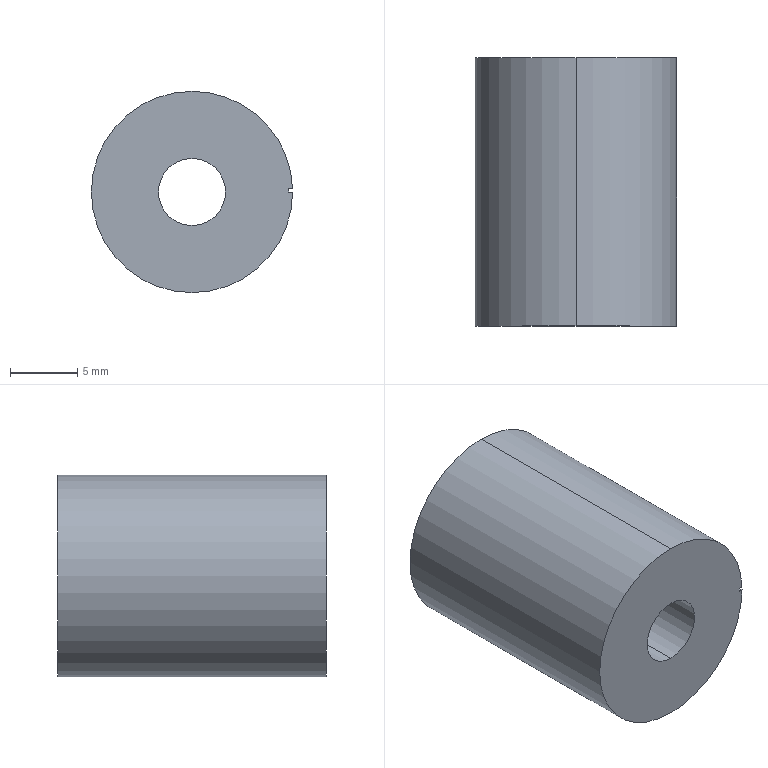Part | SolidWorks | features Extrusion 1, ICE 1 | 1 solid | 10 faces | box 15 x 20 x 15 mm | volume 3140 mm3 | cylinder 5 | plane 5 | commonest cylinder face diameters 15 x3 5 x2
STEP:
#1=CARTESIAN_POINT('',(0.,20.,-2.5));
#2=VERTEX_POINT('',#1);
#3=CARTESIAN_POINT('',(0.,20.,2.5));
#4=VERTEX_POINT('',#3);
#5=CARTESIAN_POINT('',(0.,20.,0.));
#6=DIRECTION('',(0.,1.,0.));
#7=DIRECTION('',(0.,0.,1.));
#8=AXIS2_PLACEMENT_3D('',#5,#6,#7);
#9=CIRCLE('',#8,2.5);
#10=EDGE_CURVE('',#2,#4,#9,.T.);
#11=ORIENTED_EDGE('',*,*,#10,.T.);
#12=CARTESIAN_POINT('',(0.,0.,2.5));
#13=VERTEX_POINT('',#12);
#14=CARTESIAN_POINT('',(0.,20.,2.5));
#15=DIRECTION('',(0.,-1.,0.));
#16=VECTOR('',#15,1000.);
#17=LINE('',#14,#16);
#18=EDGE_CURVE('',#4,#13,#17,.T.);
#19=ORIENTED_EDGE('',*,*,#18,.T.);
#20=CARTESIAN_POINT('',(0.,0.,-2.5));
#21=VERTEX_POINT('',#20);
#22=CARTESIAN_POINT('',(0.,0.,0.));
#23=DIRECTION('',(0.,1.,0.));
#24=DIRECTION('',(0.,0.,1.));
#25=AXIS2_PLACEMENT_3D('',#22,#23,#24);
#26=CIRCLE('',#25,2.5);
#27=EDGE_CURVE('',#21,#13,#26,.T.);
#28=ORIENTED_EDGE('',*,*,#27,.F.);
#29=CARTESIAN_POINT('',(0.,20.,-2.5));
#30=DIRECTION('',(0.,-1.,0.));
#31=VECTOR('',#30,1000.);
#32=LINE('',#29,#31);
#33=EDGE_CURVE('',#2,#21,#32,.T.);
#34=ORIENTED_EDGE('',*,*,#33,.F.);
#35=EDGE_LOOP('',(#11,#19,#28,#34));
#36=FACE_OUTER_BOUND('',#35,.T.);
#37=CARTESIAN_POINT('',(0.,20.,0.));
#38=DIRECTION('',(0.,-1.,0.));
#39=DIRECTION('',(0.,0.,-1.));
#40=AXIS2_PLACEMENT_3D('',#37,#38,#39);
#41=CYLINDRICAL_SURFACE('',#40,2.5);
#42=ADVANCED_FACE('',(#36),#41,.F.);
#43=CARTESIAN_POINT('',(0.,20.,7.5));
#44=VERTEX_POINT('',#43);
#45=CARTESIAN_POINT('',(7.496,20.,0.2452));
#46=VERTEX_POINT('',#45);
#47=CARTESIAN_POINT('',(0.,20.,0.));
#48=DIRECTION('',(0.,1.,0.));
#49=DIRECTION('',(0.,0.,1.));
#50=AXIS2_PLACEMENT_3D('',#47,#48,#49);
#51=CIRCLE('',#50,7.5);
#52=EDGE_CURVE('',#44,#46,#51,.T.);
#53=ORIENTED_EDGE('',*,*,#52,.F.);
#54=CARTESIAN_POINT('',(0.,0.,7.5));
#55=VERTEX_POINT('',#54);
#56=CARTESIAN_POINT('',(0.,20.,7.5));
#57=DIRECTION('',(0.,-1.,0.));
#58=VECTOR('',#57,1000.);
#59=LINE('',#56,#58);
#60=EDGE_CURVE('',#44,#55,#59,.T.);
#61=ORIENTED_EDGE('',*,*,#60,.T.);
#62=CARTESIAN_POINT('',(7.496,0.,0.2452));
#63=VERTEX_POINT('',#62);
#64=CARTESIAN_POINT('',(0.,0.,0.));
#65=DIRECTION('',(0.,1.,0.));
#66=DIRECTION('',(0.,0.,1.));
#67=AXIS2_PLACEMENT_3D('',#64,#65,#66);
#68=CIRCLE('',#67,7.5);
#69=EDGE_CURVE('',#55,#63,#68,.T.);
#70=ORIENTED_EDGE('',*,*,#69,.T.);
#71=CARTESIAN_POINT('',(7.496,20.,0.2452));
#72=DIRECTION('',(0.,1.,0.));
#73=VECTOR('',#72,1000.);
#74=LINE('',#71,#73);
#75=EDGE_CURVE('',#63,#46,#74,.T.);
#76=ORIENTED_EDGE('',*,*,#75,.T.);
#77=EDGE_LOOP('',(#53,#61,#70,#76));
#78=FACE_OUTER_BOUND('',#77,.T.);
#79=CARTESIAN_POINT('',(0.,20.,0.));
#80=DIRECTION('',(0.,-1.,0.));
#81=DIRECTION('',(0.,0.,-1.));
#82=AXIS2_PLACEMENT_3D('',#79,#80,#81);
#83=CYLINDRICAL_SURFACE('',#82,7.5);
#84=ADVANCED_FACE('',(#78),#83,.T.);
#85=ORIENTED_EDGE('',*,*,#60,.F.);
#86=CARTESIAN_POINT('',(0.,20.,-7.5));
#87=VERTEX_POINT('',#86);
#88=CARTESIAN_POINT('',(0.,20.,0.));
#89=DIRECTION('',(0.,1.,0.));
#90=DIRECTION('',(0.,0.,1.));
#91=AXIS2_PLACEMENT_3D('',#88,#89,#90);
#92=CIRCLE('',#91,7.5);
#93=EDGE_CURVE('',#87,#44,#92,.T.);
#94=ORIENTED_EDGE('',*,*,#93,.F.);
#95=CARTESIAN_POINT('',(0.,0.,-7.5));
#96=VERTEX_POINT('',#95);
#97=CARTESIAN_POINT('',(0.,20.,-7.5));
#98=DIRECTION('',(0.,-1.,0.));
#99=VECTOR('',#98,1000.);
#100=LINE('',#97,#99);
#101=EDGE_CURVE('',#87,#96,#100,.T.);
#102=ORIENTED_EDGE('',*,*,#101,.T.);
#103=CARTESIAN_POINT('',(0.,0.,0.));
#104=DIRECTION('',(0.,1.,0.));
#105=DIRECTION('',(0.,0.,1.));
#106=AXIS2_PLACEMENT_3D('',#103,#104,#105);
#107=CIRCLE('',#106,7.5);
#108=EDGE_CURVE('',#96,#55,#107,.T.);
#109=ORIENTED_EDGE('',*,*,#108,.T.);
#110=EDGE_LOOP('',(#85,#94,#102,#109));
#111=FACE_OUTER_BOUND('',#110,.T.);
#112=CARTESIAN_POINT('',(0.,20.,0.));
#113=DIRECTION('',(0.,-1.,0.));
#114=DIRECTION('',(0.,0.,-1.));
#115=AXIS2_PLACEMENT_3D('',#112,#113,#114);
#116=CYLINDRICAL_SURFACE('',#115,7.5);
#117=ADVANCED_FACE('',(#111),#116,.T.);
#118=CARTESIAN_POINT('',(7.198,20.,0.2452));
#119=VERTEX_POINT('',#118);
#120=CARTESIAN_POINT('',(7.198,20.,0.2452));
#121=DIRECTION('',(1.,0.,0.));
#122=VECTOR('',#121,1000.);
#123=LINE('',#120,#122);
#124=EDGE_CURVE('',#119,#46,#123,.T.);
#125=ORIENTED_EDGE('',*,*,#124,.F.);
#126=CARTESIAN_POINT('',(7.198,20.,0.));
#127=VERTEX_POINT('',#126);
#128=CARTESIAN_POINT('',(7.198,20.,0.2452));
#129=DIRECTION('',(0.,0.,1.));
#130=VECTOR('',#129,1000.);
#131=LINE('',#128,#130);
#132=EDGE_CURVE('',#127,#119,#131,.T.);
#133=ORIENTED_EDGE('',*,*,#132,.F.);
#134=CARTESIAN_POINT('',(7.5,20.,0.));
#135=VERTEX_POINT('',#134);
#136=CARTESIAN_POINT('',(7.198,20.,0.));
#137=DIRECTION('',(-1.,0.,0.));
#138=VECTOR('',#137,1000.);
#139=LINE('',#136,#138);
#140=EDGE_CURVE('',#135,#127,#139,.T.);
#141=ORIENTED_EDGE('',*,*,#140,.F.);
#142=CARTESIAN_POINT('',(0.,20.,0.));
#143=DIRECTION('',(0.,1.,0.));
#144=DIRECTION('',(0.,0.,1.));
#145=AXIS2_PLACEMENT_3D('',#142,#143,#144);
#146=CIRCLE('',#145,7.5);
#147=EDGE_CURVE('',#135,#87,#146,.T.);
#148=ORIENTED_EDGE('',*,*,#147,.T.);
#149=ORIENTED_EDGE('',*,*,#93,.T.);
#150=ORIENTED_EDGE('',*,*,#52,.T.);
#151=EDGE_LOOP('',(#125,#133,#141,#148,#149,#150));
#152=FACE_OUTER_BOUND('',#151,.T.);
#153=ORIENTED_EDGE('',*,*,#10,.F.);
#154=CARTESIAN_POINT('',(0.,20.,0.));
#155=DIRECTION('',(0.,1.,0.));
#156=DIRECTION('',(0.,0.,1.));
#157=AXIS2_PLACEMENT_3D('',#154,#155,#156);
#158=CIRCLE('',#157,2.5);
#159=EDGE_CURVE('',#4,#2,#158,.T.);
#160=ORIENTED_EDGE('',*,*,#159,.F.);
#161=EDGE_LOOP('',(#153,#160));
#162=FACE_BOUND('',#161,.T.);
#163=CARTESIAN_POINT('',(0.,20.,0.));
#164=DIRECTION('',(0.,1.,0.));
#165=DIRECTION('',(0.,0.,1.));
#166=AXIS2_PLACEMENT_3D('',#163,#164,#165);
#167=PLANE('',#166);
#168=ADVANCED_FACE('',(#152,#162),#167,.T.);
#169=CARTESIAN_POINT('',(7.198,0.,0.));
#170=VERTEX_POINT('',#169);
#171=CARTESIAN_POINT('',(7.198,0.,0.2452));
#172=VERTEX_POINT('',#171);
#173=CARTESIAN_POINT('',(7.198,0.,0.2452));
#174=DIRECTION('',(0.,0.,1.));
#175=VECTOR('',#174,1000.);
#176=LINE('',#173,#175);
#177=EDGE_CURVE('',#170,#172,#176,.T.);
#178=ORIENTED_EDGE('',*,*,#177,.T.);
#179=CARTESIAN_POINT('',(7.198,0.,0.2452));
#180=DIRECTION('',(1.,0.,0.));
#181=VECTOR('',#180,1000.);
#182=LINE('',#179,#181);
#183=EDGE_CURVE('',#172,#63,#182,.T.);
#184=ORIENTED_EDGE('',*,*,#183,.T.);
#185=ORIENTED_EDGE('',*,*,#69,.F.);
#186=ORIENTED_EDGE('',*,*,#108,.F.);
#187=CARTESIAN_POINT('',(7.5,0.,0.));
#188=VERTEX_POINT('',#187);
#189=CARTESIAN_POINT('',(0.,0.,0.));
#190=DIRECTION('',(0.,1.,0.));
#191=DIRECTION('',(0.,0.,1.));
#192=AXIS2_PLACEMENT_3D('',#189,#190,#191);
#193=CIRCLE('',#192,7.5);
#194=EDGE_CURVE('',#188,#96,#193,.T.);
#195=ORIENTED_EDGE('',*,*,#194,.F.);
#196=CARTESIAN_POINT('',(7.198,0.,0.));
#197=DIRECTION('',(-1.,0.,0.));
#198=VECTOR('',#197,1000.);
#199=LINE('',#196,#198);
#200=EDGE_CURVE('',#188,#170,#199,.T.);
#201=ORIENTED_EDGE('',*,*,#200,.T.);
#202=EDGE_LOOP('',(#178,#184,#185,#186,#195,#201));
#203=FACE_OUTER_BOUND('',#202,.T.);
#204=ORIENTED_EDGE('',*,*,#27,.T.);
#205=CARTESIAN_POINT('',(0.,0.,0.));
#206=DIRECTION('',(0.,1.,0.));
#207=DIRECTION('',(0.,0.,1.));
#208=AXIS2_PLACEMENT_3D('',#205,#206,#207);
#209=CIRCLE('',#208,2.5);
#210=EDGE_CURVE('',#13,#21,#209,.T.);
#211=ORIENTED_EDGE('',*,*,#210,.T.);
#212=EDGE_LOOP('',(#204,#211));
#213=FACE_BOUND('',#212,.T.);
#214=CARTESIAN_POINT('',(0.,0.,0.));
#215=DIRECTION('',(0.,1.,0.));
#216=DIRECTION('',(0.,0.,1.));
#217=AXIS2_PLACEMENT_3D('',#214,#215,#216);
#218=PLANE('',#217);
#219=ADVANCED_FACE('',(#203,#213),#218,.F.);
#220=ORIENTED_EDGE('',*,*,#101,.F.);
#221=ORIENTED_EDGE('',*,*,#147,.F.);
#222=CARTESIAN_POINT('',(7.5,20.,0.));
#223=DIRECTION('',(0.,-1.,0.));
#224=VECTOR('',#223,1000.);
#225=LINE('',#222,#224);
#226=EDGE_CURVE('',#135,#188,#225,.T.);
#227=ORIENTED_EDGE('',*,*,#226,.T.);
#228=ORIENTED_EDGE('',*,*,#194,.T.);
#229=EDGE_LOOP('',(#220,#221,#227,#228));
#230=FACE_OUTER_BOUND('',#229,.T.);
#231=CARTESIAN_POINT('',(0.,20.,0.));
#232=DIRECTION('',(0.,-1.,0.));
#233=DIRECTION('',(0.,0.,-1.));
#234=AXIS2_PLACEMENT_3D('',#231,#232,#233);
#235=CYLINDRICAL_SURFACE('',#234,7.5);
#236=ADVANCED_FACE('',(#230),#235,.T.);
#237=ORIENTED_EDGE('',*,*,#18,.F.);
#238=ORIENTED_EDGE('',*,*,#159,.T.);
#239=ORIENTED_EDGE('',*,*,#33,.T.);
#240=ORIENTED_EDGE('',*,*,#210,.F.);
#241=EDGE_LOOP('',(#237,#238,#239,#240));
#242=FACE_OUTER_BOUND('',#241,.T.);
#243=CARTESIAN_POINT('',(0.,20.,0.));
#244=DIRECTION('',(0.,-1.,0.));
#245=DIRECTION('',(0.,0.,-1.));
#246=AXIS2_PLACEMENT_3D('',#243,#244,#245);
#247=CYLINDRICAL_SURFACE('',#246,2.5);
#248=ADVANCED_FACE('',(#242),#247,.F.);
#249=ORIENTED_EDGE('',*,*,#183,.F.);
#250=CARTESIAN_POINT('',(7.198,0.,0.2452));
#251=DIRECTION('',(0.,1.,0.));
#252=VECTOR('',#251,1000.);
#253=LINE('',#250,#252);
#254=EDGE_CURVE('',#172,#119,#253,.T.);
#255=ORIENTED_EDGE('',*,*,#254,.T.);
#256=ORIENTED_EDGE('',*,*,#124,.T.);
#257=ORIENTED_EDGE('',*,*,#75,.F.);
#258=EDGE_LOOP('',(#249,#255,#256,#257));
#259=FACE_OUTER_BOUND('',#258,.T.);
#260=CARTESIAN_POINT('',(7.198,0.,0.2452));
#261=DIRECTION('',(0.,0.,1.));
#262=DIRECTION('',(1.,0.,0.));
#263=AXIS2_PLACEMENT_3D('',#260,#261,#262);
#264=PLANE('',#263);
#265=ADVANCED_FACE('',(#259),#264,.F.);
#266=ORIENTED_EDGE('',*,*,#140,.T.);
#267=CARTESIAN_POINT('',(7.198,0.,0.));
#268=DIRECTION('',(0.,1.,0.));
#269=VECTOR('',#268,1000.);
#270=LINE('',#267,#269);
#271=EDGE_CURVE('',#170,#127,#270,.T.);
#272=ORIENTED_EDGE('',*,*,#271,.F.);
#273=ORIENTED_EDGE('',*,*,#200,.F.);
#274=ORIENTED_EDGE('',*,*,#226,.F.);
#275=EDGE_LOOP('',(#266,#272,#273,#274));
#276=FACE_OUTER_BOUND('',#275,.T.);
#277=CARTESIAN_POINT('',(7.198,0.,0.));
#278=DIRECTION('',(0.,0.,-1.));
#279=DIRECTION('',(-1.,0.,0.));
#280=AXIS2_PLACEMENT_3D('',#277,#278,#279);
#281=PLANE('',#280);
#282=ADVANCED_FACE('',(#276),#281,.F.);
#283=ORIENTED_EDGE('',*,*,#132,.T.);
#284=ORIENTED_EDGE('',*,*,#254,.F.);
#285=ORIENTED_EDGE('',*,*,#177,.F.);
#286=ORIENTED_EDGE('',*,*,#271,.T.);
#287=EDGE_LOOP('',(#283,#284,#285,#286));
#288=FACE_OUTER_BOUND('',#287,.T.);
#289=CARTESIAN_POINT('',(7.198,0.,0.2452));
#290=DIRECTION('',(-1.,0.,0.));
#291=DIRECTION('',(0.,0.,1.));
#292=AXIS2_PLACEMENT_3D('',#289,#290,#291);
#293=PLANE('',#292);
#294=ADVANCED_FACE('',(#288),#293,.F.);
#295=CLOSED_SHELL('',(#42,#84,#117,#168,#219,#236,#248,#265,#282,#294));
#296=MANIFOLD_SOLID_BREP('',#295);
#297=CARTESIAN_POINT('',(0.,0.,0.));
#298=DIRECTION('',(0.,0.,1.));
#299=DIRECTION('',(1.,0.,0.));
#300=AXIS2_PLACEMENT_3D('',#297,#298,#299);
#301=(LENGTH_UNIT()NAMED_UNIT(*)SI_UNIT(.MILLI.,.METRE.));
#302=UNCERTAINTY_MEASURE_WITH_UNIT(LENGTH_MEASURE(0.00001),#301,'','');
#303=(NAMED_UNIT(*)PLANE_ANGLE_UNIT()SI_UNIT($,.RADIAN.));
#304=(NAMED_UNIT(*)SI_UNIT($,.STERADIAN.)SOLID_ANGLE_UNIT());
#305=(GEOMETRIC_REPRESENTATION_CONTEXT(3)GLOBAL_UNCERTAINTY_ASSIGNED_CONTEXT((#302))GLOBAL_UNIT_ASSIGNED_CONTEXT((#301,#303,#304))REPRESENTATION_CONTEXT('',''));
#306=ADVANCED_BREP_SHAPE_REPRESENTATION('',(#296,#300),#305);